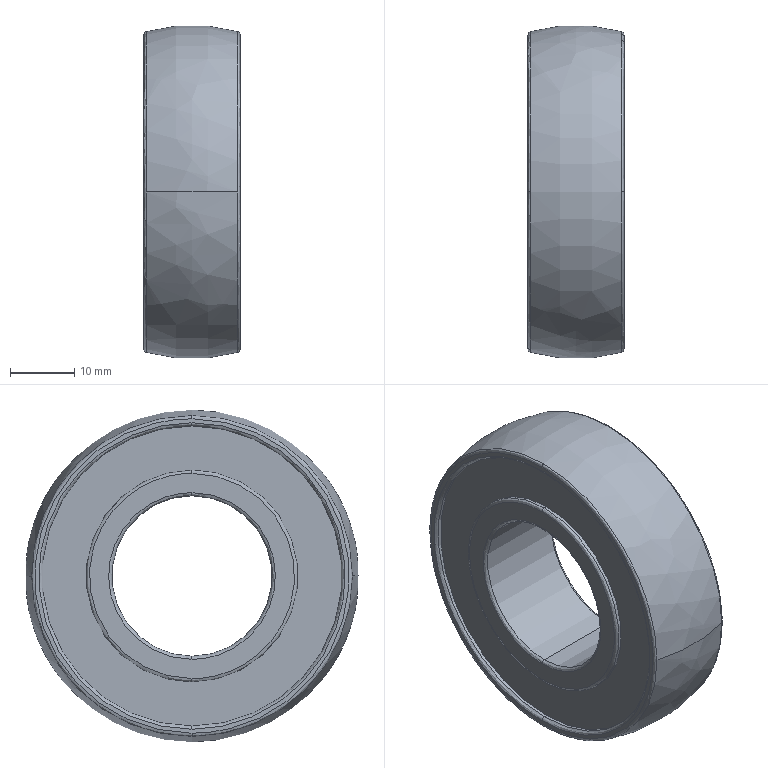Part | SolidWorks | features BaseBody 1 | 1 solid | 34 faces | box 15 x 52 x 51.979 mm | volume 21846 mm3 | spline 18 | cylinder 10 | plane 6 | commonest cylinder face diameters 33 x4 46.79 x4 25 x2